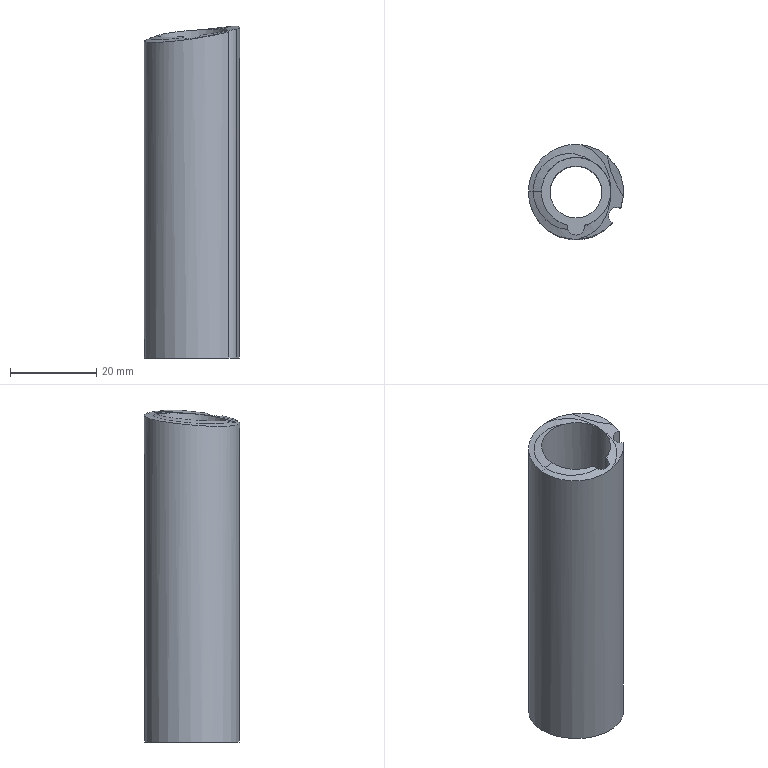Part | NX | features solid 2 | 1 solid | 14 faces | box 22 x 22.002 x 76.818 mm | volume 17878 mm3 | spline 6 | cylinder 6 | plane 2 | commonest cylinder face diameters 4 x2 12 x1 16 x1 22 x1 1640 x1
STEP:
#1=CARTESIAN_POINT('',(686.573,-10.452,-5.322));
#2=VERTEX_POINT('',#1);
#3=CARTESIAN_POINT('',(686.588,-10.686,-5.382));
#4=VERTEX_POINT('',#3);
#5=CARTESIAN_POINT('',(686.573,-10.452,-5.322));
#6=CARTESIAN_POINT('',(686.583,-10.531,-5.341));
#7=CARTESIAN_POINT('',(686.588,-10.609,-5.361));
#8=CARTESIAN_POINT('',(686.588,-10.686,-5.382));
#9=B_SPLINE_CURVE_WITH_KNOTS('',3,(#5,#6,#7,#8),.UNSPECIFIED.,.F.,.F.,(4,4),(0.00002099,0.0002621),.UNSPECIFIED.);
#10=EDGE_CURVE('',#2,#4,#9,.T.);
#11=ORIENTED_EDGE('',*,*,#10,.T.);
#12=CARTESIAN_POINT('',(686.588,-10.7,-5.386));
#13=VERTEX_POINT('',#12);
#14=CARTESIAN_POINT('',(686.588,-10.686,-5.382));
#15=CARTESIAN_POINT('',(686.588,-10.691,-5.383));
#16=CARTESIAN_POINT('',(686.588,-10.695,-5.385));
#17=CARTESIAN_POINT('',(686.588,-10.7,-5.386));
#18=B_SPLINE_CURVE_WITH_KNOTS('',3,(#14,#15,#16,#17),.UNSPECIFIED.,.F.,.F.,(4,4),(0.005452,0.005466),.UNSPECIFIED.);
#19=EDGE_CURVE('',#4,#13,#18,.T.);
#20=ORIENTED_EDGE('',*,*,#19,.T.);
#21=CARTESIAN_POINT('',(687.707,-10.069,-5.195));
#22=VERTEX_POINT('',#21);
#23=CARTESIAN_POINT('',(687.707,-10.069,-5.195));
#24=CARTESIAN_POINT('',(687.355,-10.307,-5.258));
#25=CARTESIAN_POINT('',(686.981,-10.519,-5.322));
#26=CARTESIAN_POINT('',(686.588,-10.7,-5.386));
#27=B_SPLINE_CURVE_WITH_KNOTS('',3,(#23,#24,#25,#26),.UNSPECIFIED.,.F.,.F.,(4,4),(0.3466,0.3956),.UNSPECIFIED.);
#28=EDGE_CURVE('',#22,#13,#27,.T.);
#29=ORIENTED_EDGE('',*,*,#28,.F.);
#30=CARTESIAN_POINT('',(687.707,-10.069,-5.195));
#31=CARTESIAN_POINT('',(687.34,-10.225,-5.239));
#32=CARTESIAN_POINT('',(686.962,-10.353,-5.281));
#33=CARTESIAN_POINT('',(686.573,-10.452,-5.322));
#34=B_SPLINE_CURVE_WITH_KNOTS('',3,(#30,#31,#32,#33),.UNSPECIFIED.,.F.,.F.,(4,4),(0.009294,0.0105),.UNSPECIFIED.);
#35=EDGE_CURVE('',#22,#2,#34,.T.);
#36=ORIENTED_EDGE('',*,*,#35,.T.);
#37=EDGE_LOOP('',(#11,#20,#29,#36));
#38=FACE_BOUND('',#37,.T.);
#39=CARTESIAN_POINT('',(686.515,-10.456,-5.325));
#40=CARTESIAN_POINT('',(686.529,-10.505,-5.337));
#41=CARTESIAN_POINT('',(686.542,-10.555,-5.349));
#42=CARTESIAN_POINT('',(686.555,-10.604,-5.361));
#43=CARTESIAN_POINT('',(686.568,-10.654,-5.374));
#44=CARTESIAN_POINT('',(686.581,-10.703,-5.387));
#45=CARTESIAN_POINT('',(686.761,-10.397,-5.3));
#46=CARTESIAN_POINT('',(686.775,-10.446,-5.311));
#47=CARTESIAN_POINT('',(686.79,-10.495,-5.323));
#48=CARTESIAN_POINT('',(686.805,-10.544,-5.336));
#49=CARTESIAN_POINT('',(686.82,-10.593,-5.348));
#50=CARTESIAN_POINT('',(686.834,-10.642,-5.361));
#51=CARTESIAN_POINT('',(687.004,-10.328,-5.274));
#52=CARTESIAN_POINT('',(687.02,-10.377,-5.286));
#53=CARTESIAN_POINT('',(687.036,-10.426,-5.297));
#54=CARTESIAN_POINT('',(687.053,-10.474,-5.309));
#55=CARTESIAN_POINT('',(687.069,-10.523,-5.322));
#56=CARTESIAN_POINT('',(687.085,-10.571,-5.335));
#57=CARTESIAN_POINT('',(687.244,-10.25,-5.248));
#58=CARTESIAN_POINT('',(687.261,-10.298,-5.259));
#59=CARTESIAN_POINT('',(687.279,-10.346,-5.271));
#60=CARTESIAN_POINT('',(687.297,-10.394,-5.283));
#61=CARTESIAN_POINT('',(687.315,-10.443,-5.295));
#62=CARTESIAN_POINT('',(687.333,-10.49,-5.307));
#63=CARTESIAN_POINT('',(687.48,-10.162,-5.221));
#64=CARTESIAN_POINT('',(687.5,-10.21,-5.232));
#65=CARTESIAN_POINT('',(687.519,-10.257,-5.244));
#66=CARTESIAN_POINT('',(687.538,-10.305,-5.255));
#67=CARTESIAN_POINT('',(687.558,-10.352,-5.267));
#68=CARTESIAN_POINT('',(687.577,-10.4,-5.28));
#69=CARTESIAN_POINT('',(687.713,-10.065,-5.194));
#70=CARTESIAN_POINT('',(687.734,-10.112,-5.205));
#71=CARTESIAN_POINT('',(687.755,-10.159,-5.216));
#72=CARTESIAN_POINT('',(687.776,-10.206,-5.228));
#73=CARTESIAN_POINT('',(687.797,-10.253,-5.24));
#74=CARTESIAN_POINT('',(687.818,-10.3,-5.252));
#75=B_SPLINE_SURFACE_WITH_KNOTS('',5,5,((#39,#40,#41,#42,#43,#44),(#45,#46,#47,#48,#49,#50),(#51,#52,#53,#54,#55,#56),(#57,#58,#59,#60,#61,#62),(#63,#64,#65,#66,#67,#68),(#69,#70,#71,#72,#73,#74)),.UNSPECIFIED.,.F.,.F.,.F.,(6,6),(6,6),(0.5791,0.6294),(0.4469,0.5178),.PIECEWISE_BEZIER_KNOTS.);
#76=ADVANCED_FACE('',(#38),#75,.F.);
#77=CARTESIAN_POINT('',(692.961,-9.836,-4.56));
#78=VERTEX_POINT('',#77);
#79=CARTESIAN_POINT('',(692.961,-9.836,-80.));
#80=VERTEX_POINT('',#79);
#81=CARTESIAN_POINT('',(692.961,-9.836,170.));
#82=DIRECTION('',(0.,0.,-1.));
#83=VECTOR('',#82,1000.);
#84=LINE('',#81,#83);
#85=EDGE_CURVE('',#78,#80,#84,.T.);
#86=ORIENTED_EDGE('',*,*,#85,.F.);
#87=CARTESIAN_POINT('',(684.901,-13.701,-6.131));
#88=VERTEX_POINT('',#87);
#89=CARTESIAN_POINT('',(684.948,-13.696,-6.124));
#90=CARTESIAN_POINT('',(688.008,-13.596,-5.653));
#91=CARTESIAN_POINT('',(690.985,-12.155,-5.066));
#92=CARTESIAN_POINT('',(692.961,-9.836,-4.56));
#93=B_SPLINE_CURVE_WITH_KNOTS('',3,(#89,#90,#91,#92),.UNSPECIFIED.,.F.,.F.,(4,4),(0.01762,0.02686),.UNSPECIFIED.);
#94=EDGE_CURVE('',#88,#78,#93,.T.);
#95=ORIENTED_EDGE('',*,*,#94,.F.);
#96=CARTESIAN_POINT('',(673.59,-2.498,-6.658));
#97=VERTEX_POINT('',#96);
#98=CARTESIAN_POINT('',(673.59,-2.498,-6.658));
#99=CARTESIAN_POINT('',(673.535,-5.487,-6.917));
#100=CARTESIAN_POINT('',(675.984,-11.422,-7.155));
#101=CARTESIAN_POINT('',(681.928,-13.779,-6.586));
#102=CARTESIAN_POINT('',(684.89,-13.698,-6.132));
#103=B_SPLINE_CURVE_WITH_KNOTS('',3,(#98,#99,#100,#101,#102),.UNSPECIFIED.,.F.,.F.,(4,1,4),(0.,0.008898,0.0178),.UNSPECIFIED.);
#104=EDGE_CURVE('',#97,#88,#103,.T.);
#105=ORIENTED_EDGE('',*,*,#104,.F.);
#106=CARTESIAN_POINT('',(685.747,8.237,-4.236));
#107=VERTEX_POINT('',#106);
#108=CARTESIAN_POINT('',(673.59,-2.498,-6.658));
#109=CARTESIAN_POINT('',(673.647,0.5842,-6.392));
#110=CARTESIAN_POINT('',(676.467,6.538,-5.598));
#111=CARTESIAN_POINT('',(682.699,8.559,-4.676));
#112=CARTESIAN_POINT('',(685.745,8.237,-4.237));
#113=B_SPLINE_CURVE_WITH_KNOTS('',3,(#108,#109,#110,#111,#112),.UNSPECIFIED.,.F.,.F.,(4,1,4),(0.,0.009181,0.01836),.UNSPECIFIED.);
#114=EDGE_CURVE('',#97,#107,#113,.T.);
#115=ORIENTED_EDGE('',*,*,#114,.T.);
#116=CARTESIAN_POINT('',(691.785,5.616,-3.502));
#117=VERTEX_POINT('',#116);
#118=CARTESIAN_POINT('',(691.783,5.619,-3.503));
#119=CARTESIAN_POINT('',(690.087,7.085,-3.656));
#120=CARTESIAN_POINT('',(687.953,8.002,-3.918));
#121=CARTESIAN_POINT('',(685.754,8.236,-4.235));
#122=B_SPLINE_CURVE_WITH_KNOTS('',3,(#118,#119,#120,#121),.UNSPECIFIED.,.F.,.F.,(4,4),(0.04406,0.05075),.UNSPECIFIED.);
#123=EDGE_CURVE('',#117,#107,#122,.T.);
#124=ORIENTED_EDGE('',*,*,#123,.F.);
#125=CARTESIAN_POINT('',(695.532,-3.818,-3.655));
#126=VERTEX_POINT('',#125);
#127=CARTESIAN_POINT('',(691.788,5.614,-3.502));
#128=CARTESIAN_POINT('',(693.13,4.452,-3.381));
#129=CARTESIAN_POINT('',(695.206,1.508,-2.937));
#130=CARTESIAN_POINT('',(695.711,-2.052,-3.483));
#131=CARTESIAN_POINT('',(695.532,-3.814,-3.655));
#132=B_SPLINE_CURVE_WITH_KNOTS('',3,(#127,#128,#129,#130,#131),.UNSPECIFIED.,.F.,.F.,(4,1,4),(0.,0.005263,0.01053),.UNSPECIFIED.);
#133=EDGE_CURVE('',#117,#126,#132,.T.);
#134=ORIENTED_EDGE('',*,*,#133,.T.);
#135=CARTESIAN_POINT('',(694.953,-6.386,-3.958));
#136=VERTEX_POINT('',#135);
#137=CARTESIAN_POINT('',(694.953,-6.386,-3.958));
#138=CARTESIAN_POINT('',(695.246,-5.562,-3.843));
#139=CARTESIAN_POINT('',(695.441,-4.706,-3.742));
#140=CARTESIAN_POINT('',(695.531,-3.822,-3.655));
#141=B_SPLINE_CURVE_WITH_KNOTS('',3,(#137,#138,#139,#140),.UNSPECIFIED.,.F.,.F.,(4,4),(0.03089,0.03354),.UNSPECIFIED.);
#142=EDGE_CURVE('',#136,#126,#141,.T.);
#143=ORIENTED_EDGE('',*,*,#142,.F.);
#144=CARTESIAN_POINT('',(694.953,-6.386,-80.));
#145=VERTEX_POINT('',#144);
#146=CARTESIAN_POINT('',(694.953,-6.386,170.));
#147=DIRECTION('',(0.,0.,-1.));
#148=VECTOR('',#147,1000.);
#149=LINE('',#146,#148);
#150=EDGE_CURVE('',#145,#136,#149,.F.);
#151=ORIENTED_EDGE('',*,*,#150,.F.);
#152=CARTESIAN_POINT('',(684.588,-2.702,-80.));
#153=DIRECTION('',(0.,0.,1.));
#154=DIRECTION('',(1.,0.,0.));
#155=AXIS2_PLACEMENT_3D('',#152,#153,#154);
#156=CIRCLE('',#155,11.);
#157=EDGE_CURVE('',#145,#80,#156,.T.);
#158=ORIENTED_EDGE('',*,*,#157,.T.);
#159=EDGE_LOOP('',(#86,#95,#105,#115,#124,#134,#143,#151,#158));
#160=FACE_BOUND('',#159,.T.);
#161=CARTESIAN_POINT('',(684.588,-2.702,27.));
#162=DIRECTION('',(0.,0.,-1.));
#163=DIRECTION('',(-1.,0.,0.));
#164=AXIS2_PLACEMENT_3D('',#161,#162,#163);
#165=CYLINDRICAL_SURFACE('',#164,11.);
#166=ADVANCED_FACE('',(#160),#165,.T.);
#167=CARTESIAN_POINT('',(690.588,-2.702,-80.));
#168=VERTEX_POINT('',#167);
#169=CARTESIAN_POINT('',(684.588,-2.702,-80.));
#170=DIRECTION('',(0.,0.,1.));
#171=DIRECTION('',(1.,0.,0.));
#172=AXIS2_PLACEMENT_3D('',#169,#170,#171);
#173=CIRCLE('',#172,6.);
#174=EDGE_CURVE('',#168,#168,#173,.T.);
#175=ORIENTED_EDGE('',*,*,#174,.T.);
#176=EDGE_LOOP('',(#175));
#177=FACE_BOUND('',#176,.T.);
#178=CARTESIAN_POINT('',(694.115,-8.202,-80.));
#179=DIRECTION('',(0.,0.,1.));
#180=DIRECTION('',(0.866,-0.5,0.));
#181=AXIS2_PLACEMENT_3D('',#178,#179,#180);
#182=CIRCLE('',#181,2.);
#183=EDGE_CURVE('',#145,#80,#182,.T.);
#184=ORIENTED_EDGE('',*,*,#183,.T.);
#185=ORIENTED_EDGE('',*,*,#157,.F.);
#186=EDGE_LOOP('',(#184,#185));
#187=FACE_BOUND('',#186,.T.);
#188=CARTESIAN_POINT('',(-628.999,-86.749,-80.));
#189=DIRECTION('',(0.,0.,1.));
#190=DIRECTION('',(1.,0.,0.));
#191=AXIS2_PLACEMENT_3D('',#188,#189,#190);
#192=PLANE('',#191);
#193=ADVANCED_FACE('',(#177,#187),#192,.F.);
#194=ORIENTED_EDGE('',*,*,#94,.T.);
#195=CARTESIAN_POINT('',(692.961,-9.836,-4.56));
#196=CARTESIAN_POINT('',(692.558,-9.552,-4.602));
#197=CARTESIAN_POINT('',(691.968,-8.66,-4.625));
#198=CARTESIAN_POINT('',(692.228,-7.09,-4.457));
#199=CARTESIAN_POINT('',(693.458,-6.116,-4.18));
#200=CARTESIAN_POINT('',(694.506,-6.18,-4.014));
#201=CARTESIAN_POINT('',(694.953,-6.386,-3.958));
#202=B_SPLINE_CURVE_WITH_KNOTS('',3,(#195,#196,#197,#198,#199,#200,#201),.UNSPECIFIED.,.F.,.F.,(4,1,1,1,4),(0.003125,0.00461,0.006094,0.007579,0.009063),.UNSPECIFIED.);
#203=EDGE_CURVE('',#78,#136,#202,.T.);
#204=ORIENTED_EDGE('',*,*,#203,.T.);
#205=ORIENTED_EDGE('',*,*,#142,.T.);
#206=CARTESIAN_POINT('',(691.783,5.616,-3.503));
#207=CARTESIAN_POINT('',(692.343,2.264,-3.684));
#208=CARTESIAN_POINT('',(693.654,-1.017,-3.738));
#209=CARTESIAN_POINT('',(695.53,-3.82,-3.656));
#210=B_SPLINE_CURVE_WITH_KNOTS('',3,(#206,#207,#208,#209),.UNSPECIFIED.,.F.,.F.,(4,4),(0.1057,0.3726),.UNSPECIFIED.);
#211=EDGE_CURVE('',#126,#117,#210,.F.);
#212=ORIENTED_EDGE('',*,*,#211,.T.);
#213=ORIENTED_EDGE('',*,*,#123,.T.);
#214=CARTESIAN_POINT('',(692.623,-2.801,-4.047));
#215=VERTEX_POINT('',#214);
#216=CARTESIAN_POINT('',(685.75,8.237,-4.236));
#217=CARTESIAN_POINT('',(686.39,8.019,-4.156));
#218=CARTESIAN_POINT('',(687.294,7.605,-4.05));
#219=CARTESIAN_POINT('',(688.457,6.826,-3.932));
#220=CARTESIAN_POINT('',(689.404,6.048,-3.846));
#221=CARTESIAN_POINT('',(690.246,5.136,-3.787));
#222=CARTESIAN_POINT('',(690.868,4.228,-3.761));
#223=CARTESIAN_POINT('',(691.181,3.695,-3.754));
#224=CARTESIAN_POINT('',(691.498,3.099,-3.751));
#225=CARTESIAN_POINT('',(691.949,2.052,-3.764));
#226=CARTESIAN_POINT('',(692.483,0.08758,-3.836));
#227=CARTESIAN_POINT('',(692.637,-1.596,-3.948));
#228=CARTESIAN_POINT('',(692.623,-2.801,-4.047));
#229=B_SPLINE_CURVE_WITH_KNOTS('',3,(#216,#217,#218,#219,#220,#221,#222,#223,#224,#225,#226,#227,#228),.UNSPECIFIED.,.F.,.F.,(4,1,1,1,1,1,1,1,1,1,4),(0.5367,0.5946,0.6236,0.6525,0.7104,0.7394,0.7539,0.7683,0.8263,0.8842,1.),.UNSPECIFIED.);
#230=EDGE_CURVE('',#107,#215,#229,.T.);
#231=ORIENTED_EDGE('',*,*,#230,.T.);
#232=CARTESIAN_POINT('',(684.912,-13.704,-6.13));
#233=CARTESIAN_POINT('',(685.602,-13.549,-6.013));
#234=CARTESIAN_POINT('',(686.915,-13.103,-5.777));
#235=CARTESIAN_POINT('',(688.718,-11.987,-5.408));
#236=CARTESIAN_POINT('',(689.847,-10.911,-5.144));
#237=CARTESIAN_POINT('',(690.532,-10.04,-4.965));
#238=CARTESIAN_POINT('',(690.902,-9.484,-4.862));
#239=CARTESIAN_POINT('',(691.19,-9.002,-4.777));
#240=CARTESIAN_POINT('',(691.46,-8.481,-4.692));
#241=CARTESIAN_POINT('',(691.867,-7.54,-4.551));
#242=CARTESIAN_POINT('',(692.408,-5.789,-4.323));
#243=CARTESIAN_POINT('',(692.609,-4.055,-4.15));
#244=CARTESIAN_POINT('',(692.623,-2.801,-4.047));
#245=B_SPLINE_CURVE_WITH_KNOTS('',3,(#232,#233,#234,#235,#236,#237,#238,#239,#240,#241,#242,#243,#244),.UNSPECIFIED.,.F.,.F.,(4,1,1,1,1,1,1,1,1,1,4),(0.5156,0.5762,0.6367,0.6973,0.7275,0.7427,0.7578,0.7881,0.8184,0.8789,1.),.UNSPECIFIED.);
#246=EDGE_CURVE('',#88,#215,#245,.T.);
#247=ORIENTED_EDGE('',*,*,#246,.F.);
#248=EDGE_LOOP('',(#194,#204,#205,#212,#213,#231,#247));
#249=FACE_BOUND('',#248,.T.);
#250=CARTESIAN_POINT('',(561.704,-30.67,805.818));
#251=DIRECTION('',(0.02304,-0.9968,-0.07674));
#252=DIRECTION('',(0.9976,0.02799,-0.06404));
#253=AXIS2_PLACEMENT_3D('',#250,#251,#252);
#254=CYLINDRICAL_SURFACE('',#253,820.);
#255=ADVANCED_FACE('',(#249),#254,.F.);
#256=ORIENTED_EDGE('',*,*,#211,.F.);
#257=ORIENTED_EDGE('',*,*,#133,.F.);
#258=EDGE_LOOP('',(#256,#257));
#259=FACE_BOUND('',#258,.T.);
#260=CARTESIAN_POINT('',(695.568,-3.868,-3.653));
#261=CARTESIAN_POINT('',(695.914,-3.635,-3.577));
#262=CARTESIAN_POINT('',(696.256,-3.405,-3.479));
#263=CARTESIAN_POINT('',(696.594,-3.177,-3.36));
#264=CARTESIAN_POINT('',(696.925,-2.952,-3.219));
#265=CARTESIAN_POINT('',(697.249,-2.732,-3.057));
#266=CARTESIAN_POINT('',(694.938,-2.931,-3.681));
#267=CARTESIAN_POINT('',(695.294,-2.716,-3.606));
#268=CARTESIAN_POINT('',(695.647,-2.503,-3.508));
#269=CARTESIAN_POINT('',(695.995,-2.292,-3.388));
#270=CARTESIAN_POINT('',(696.336,-2.085,-3.248));
#271=CARTESIAN_POINT('',(696.67,-1.882,-3.086));
#272=CARTESIAN_POINT('',(694.361,-1.956,-3.697));
#273=CARTESIAN_POINT('',(694.727,-1.759,-3.621));
#274=CARTESIAN_POINT('',(695.089,-1.564,-3.524));
#275=CARTESIAN_POINT('',(695.446,-1.371,-3.405));
#276=CARTESIAN_POINT('',(695.797,-1.181,-3.265));
#277=CARTESIAN_POINT('',(696.14,-0.9951,-3.104));
#278=CARTESIAN_POINT('',(693.842,-0.9469,-3.7));
#279=CARTESIAN_POINT('',(694.215,-0.7679,-3.625));
#280=CARTESIAN_POINT('',(694.586,-0.5907,-3.528));
#281=CARTESIAN_POINT('',(694.951,-0.4159,-3.409));
#282=CARTESIAN_POINT('',(695.31,-0.2441,-3.27));
#283=CARTESIAN_POINT('',(695.662,-0.07604,-3.11));
#284=CARTESIAN_POINT('',(693.03,0.8862,-3.684));
#285=CARTESIAN_POINT('',(693.417,1.032,-3.609));
#286=CARTESIAN_POINT('',(693.8,1.177,-3.513));
#287=CARTESIAN_POINT('',(694.179,1.319,-3.396));
#288=CARTESIAN_POINT('',(694.55,1.459,-3.258));
#289=CARTESIAN_POINT('',(694.915,1.595,-3.099));
#290=CARTESIAN_POINT('',(692.413,2.795,-3.629));
#291=CARTESIAN_POINT('',(692.809,2.908,-3.556));
#292=CARTESIAN_POINT('',(693.202,3.019,-3.462));
#293=CARTESIAN_POINT('',(693.59,3.128,-3.346));
#294=CARTESIAN_POINT('',(693.971,3.234,-3.21));
#295=CARTESIAN_POINT('',(694.345,3.337,-3.053));
#296=CARTESIAN_POINT('',(692.182,3.634,-3.599));
#297=CARTESIAN_POINT('',(692.582,3.732,-3.526));
#298=CARTESIAN_POINT('',(692.979,3.829,-3.433));
#299=CARTESIAN_POINT('',(693.37,3.923,-3.318));
#300=CARTESIAN_POINT('',(693.755,4.015,-3.182));
#301=CARTESIAN_POINT('',(694.133,4.104,-3.026));
#302=CARTESIAN_POINT('',(691.975,4.55,-3.558));
#303=CARTESIAN_POINT('',(692.378,4.632,-3.487));
#304=CARTESIAN_POINT('',(692.778,4.712,-3.394));
#305=CARTESIAN_POINT('',(693.172,4.791,-3.28));
#306=CARTESIAN_POINT('',(693.561,4.867,-3.145));
#307=CARTESIAN_POINT('',(693.942,4.94,-2.99));
#308=CARTESIAN_POINT('',(691.812,5.474,-3.51));
#309=CARTESIAN_POINT('',(692.218,5.54,-3.439));
#310=CARTESIAN_POINT('',(692.62,5.604,-3.347));
#311=CARTESIAN_POINT('',(693.017,5.667,-3.235));
#312=CARTESIAN_POINT('',(693.408,5.727,-3.101));
#313=CARTESIAN_POINT('',(693.791,5.785,-2.947));
#314=CARTESIAN_POINT('',(691.8,5.542,-3.506));
#315=CARTESIAN_POINT('',(692.206,5.607,-3.436));
#316=CARTESIAN_POINT('',(692.609,5.67,-3.344));
#317=CARTESIAN_POINT('',(693.006,5.731,-3.231));
#318=CARTESIAN_POINT('',(693.397,5.79,-3.098));
#319=CARTESIAN_POINT('',(693.781,5.847,-2.944));
#320=CARTESIAN_POINT('',(691.789,5.61,-3.502));
#321=CARTESIAN_POINT('',(692.195,5.673,-3.432));
#322=CARTESIAN_POINT('',(692.597,5.735,-3.34));
#323=CARTESIAN_POINT('',(692.995,5.795,-3.228));
#324=CARTESIAN_POINT('',(693.386,5.853,-3.094));
#325=CARTESIAN_POINT('',(693.77,5.909,-2.941));
#326=CARTESIAN_POINT('',(691.778,5.678,-3.499));
#327=CARTESIAN_POINT('',(692.184,5.74,-3.429));
#328=CARTESIAN_POINT('',(692.587,5.801,-3.337));
#329=CARTESIAN_POINT('',(692.984,5.86,-3.224));
#330=CARTESIAN_POINT('',(693.376,5.916,-3.091));
#331=CARTESIAN_POINT('',(693.76,5.971,-2.937));
#332=B_SPLINE_SURFACE_WITH_KNOTS('',5,5,((#260,#261,#262,#263,#264,#265),(#266,#267,#268,#269,#270,#271),(#272,#273,#274,#275,#276,#277),(#278,#279,#280,#281,#282,#283),(#284,#285,#286,#287,#288,#289),(#290,#291,#292,#293,#294,#295),(#296,#297,#298,#299,#300,#301),(#302,#303,#304,#305,#306,#307),(#308,#309,#310,#311,#312,#313),(#314,#315,#316,#317,#318,#319),(#320,#321,#322,#323,#324,#325),(#326,#327,#328,#329,#330,#331)),.UNSPECIFIED.,.F.,.F.,.F.,(6,3,3,6),(6,6),(0.6261,0.7739,0.887,0.8959),(0.,0.4938),.UNSPECIFIED.);
#333=ADVANCED_FACE('',(#259),#332,.F.);
#334=CARTESIAN_POINT('',(674.688,-2.535,-6.203));
#335=VERTEX_POINT('',#334);
#336=CARTESIAN_POINT('',(674.688,-2.535,-6.203));
#337=CARTESIAN_POINT('',(674.331,-2.521,-6.376));
#338=CARTESIAN_POINT('',(673.965,-2.509,-6.528));
#339=CARTESIAN_POINT('',(673.59,-2.498,-6.658));
#340=B_SPLINE_CURVE_WITH_KNOTS('',3,(#336,#337,#338,#339),.UNSPECIFIED.,.F.,.F.,(4,4),(0.,0.3711),.UNSPECIFIED.);
#341=EDGE_CURVE('',#335,#97,#340,.T.);
#342=ORIENTED_EDGE('',*,*,#341,.F.);
#343=CARTESIAN_POINT('',(687.878,4.59,-3.984));
#344=VERTEX_POINT('',#343);
#345=CARTESIAN_POINT('',(687.878,4.59,-3.984));
#346=CARTESIAN_POINT('',(686.719,5.44,-4.06));
#347=CARTESIAN_POINT('',(683.861,6.559,-4.333));
#348=CARTESIAN_POINT('',(679.15,5.648,-5.001));
#349=CARTESIAN_POINT('',(675.576,2.281,-5.709));
#350=CARTESIAN_POINT('',(674.69,-0.9257,-6.073));
#351=CARTESIAN_POINT('',(674.688,-2.535,-6.203));
#352=B_SPLINE_CURVE_WITH_KNOTS('',3,(#345,#346,#347,#348,#349,#350,#351),.UNSPECIFIED.,.F.,.F.,(4,1,1,1,4),(0.3426,0.5069,0.6713,0.8356,1.),.UNSPECIFIED.);
#353=EDGE_CURVE('',#344,#335,#352,.T.);
#354=ORIENTED_EDGE('',*,*,#353,.F.);
#355=CARTESIAN_POINT('',(692.588,-2.8,-4.053));
#356=VERTEX_POINT('',#355);
#357=CARTESIAN_POINT('',(687.878,4.59,-3.984));
#358=CARTESIAN_POINT('',(689.299,3.949,-3.92));
#359=CARTESIAN_POINT('',(691.711,1.852,-3.826));
#360=CARTESIAN_POINT('',(692.607,-1.245,-3.924));
#361=CARTESIAN_POINT('',(692.588,-2.8,-4.053));
#362=B_SPLINE_CURVE_WITH_KNOTS('',3,(#357,#358,#359,#360,#361),.UNSPECIFIED.,.F.,.F.,(4,1,4),(0.,0.004613,0.009227),.UNSPECIFIED.);
#363=EDGE_CURVE('',#344,#356,#362,.T.);
#364=ORIENTED_EDGE('',*,*,#363,.T.);
#365=CARTESIAN_POINT('',(692.623,-2.801,-4.047));
#366=CARTESIAN_POINT('',(692.611,-2.8,-4.049));
#367=CARTESIAN_POINT('',(692.6,-2.8,-4.051));
#368=CARTESIAN_POINT('',(692.588,-2.8,-4.053));
#369=B_SPLINE_CURVE_WITH_KNOTS('',3,(#365,#366,#367,#368),.UNSPECIFIED.,.F.,.F.,(4,4),(0.,0.02906),.UNSPECIFIED.);
#370=EDGE_CURVE('',#215,#356,#369,.T.);
#371=ORIENTED_EDGE('',*,*,#370,.F.);
#372=ORIENTED_EDGE('',*,*,#230,.F.);
#373=ORIENTED_EDGE('',*,*,#114,.F.);
#374=EDGE_LOOP('',(#342,#354,#364,#371,#372,#373));
#375=FACE_BOUND('',#374,.T.);
#376=CARTESIAN_POINT('',(671.633,-2.461,-7.124));
#377=CARTESIAN_POINT('',(672.268,-2.468,-7.039));
#378=CARTESIAN_POINT('',(672.897,-2.479,-6.903));
#379=CARTESIAN_POINT('',(673.513,-2.494,-6.717));
#380=CARTESIAN_POINT('',(674.112,-2.513,-6.483));
#381=CARTESIAN_POINT('',(674.688,-2.535,-6.203));
#382=CARTESIAN_POINT('',(671.634,-1.201,-7.023));
#383=CARTESIAN_POINT('',(672.269,-1.276,-6.943));
#384=CARTESIAN_POINT('',(672.898,-1.356,-6.813));
#385=CARTESIAN_POINT('',(673.514,-1.439,-6.632));
#386=CARTESIAN_POINT('',(674.113,-1.524,-6.403));
#387=CARTESIAN_POINT('',(674.689,-1.612,-6.128));
#388=CARTESIAN_POINT('',(671.804,0.0567,-6.899));
#389=CARTESIAN_POINT('',(672.429,-0.08687,-6.826));
#390=CARTESIAN_POINT('',(673.047,-0.2345,-6.703));
#391=CARTESIAN_POINT('',(673.653,-0.3849,-6.529));
#392=CARTESIAN_POINT('',(674.242,-0.5369,-6.308));
#393=CARTESIAN_POINT('',(674.808,-0.6891,-6.04));
#394=CARTESIAN_POINT('',(672.143,1.281,-6.755));
#395=CARTESIAN_POINT('',(672.747,1.071,-6.69));
#396=CARTESIAN_POINT('',(673.344,0.8575,-6.575));
#397=CARTESIAN_POINT('',(673.93,0.6416,-6.41));
#398=CARTESIAN_POINT('',(674.498,0.4254,-6.198));
#399=CARTESIAN_POINT('',(675.045,0.2106,-5.939));
#400=CARTESIAN_POINT('',(673.582,4.609,-6.294));
#401=CARTESIAN_POINT('',(674.097,4.223,-6.254));
#402=CARTESIAN_POINT('',(674.605,3.833,-6.166));
#403=CARTESIAN_POINT('',(675.102,3.442,-6.03));
#404=CARTESIAN_POINT('',(675.585,3.054,-5.847));
#405=CARTESIAN_POINT('',(676.049,2.671,-5.62));
#406=CARTESIAN_POINT('',(676.202,7.164,-5.726));
#407=CARTESIAN_POINT('',(676.558,6.655,-5.717));
#408=CARTESIAN_POINT('',(676.907,6.141,-5.663));
#409=CARTESIAN_POINT('',(677.247,5.629,-5.565));
#410=CARTESIAN_POINT('',(677.576,5.12,-5.422));
#411=CARTESIAN_POINT('',(677.891,4.619,-5.238));
#412=CARTESIAN_POINT('',(678.304,8.32,-5.337));
#413=CARTESIAN_POINT('',(678.534,7.765,-5.348));
#414=CARTESIAN_POINT('',(678.758,7.206,-5.317));
#415=CARTESIAN_POINT('',(678.974,6.649,-5.245));
#416=CARTESIAN_POINT('',(679.182,6.095,-5.132));
#417=CARTESIAN_POINT('',(679.379,5.55,-4.979));
#418=CARTESIAN_POINT('',(682.432,9.268,-4.659));
#419=CARTESIAN_POINT('',(682.43,8.708,-4.704));
#420=CARTESIAN_POINT('',(682.423,8.145,-4.713));
#421=CARTESIAN_POINT('',(682.411,7.582,-4.687));
#422=CARTESIAN_POINT('',(682.394,7.023,-4.625));
#423=CARTESIAN_POINT('',(682.372,6.471,-4.529));
#424=CARTESIAN_POINT('',(686.302,8.282,-4.151));
#425=CARTESIAN_POINT('',(686.119,7.828,-4.215));
#426=CARTESIAN_POINT('',(685.932,7.372,-4.251));
#427=CARTESIAN_POINT('',(685.742,6.916,-4.258));
#428=CARTESIAN_POINT('',(685.549,6.461,-4.237));
#429=CARTESIAN_POINT('',(685.354,6.011,-4.187));
#430=CARTESIAN_POINT('',(687.873,7.465,-3.973));
#431=CARTESIAN_POINT('',(687.628,7.078,-4.042));
#432=CARTESIAN_POINT('',(687.379,6.689,-4.086));
#433=CARTESIAN_POINT('',(687.127,6.299,-4.105));
#434=CARTESIAN_POINT('',(686.873,5.911,-4.098));
#435=CARTESIAN_POINT('',(686.619,5.525,-4.065));
#436=CARTESIAN_POINT('',(689.86,5.811,-3.794));
#437=CARTESIAN_POINT('',(689.558,5.537,-3.864));
#438=CARTESIAN_POINT('',(689.253,5.26,-3.913));
#439=CARTESIAN_POINT('',(688.946,4.983,-3.943));
#440=CARTESIAN_POINT('',(688.638,4.706,-3.951));
#441=CARTESIAN_POINT('',(688.33,4.43,-3.939));
#442=CARTESIAN_POINT('',(691.158,3.833,-3.747));
#443=CARTESIAN_POINT('',(690.849,3.66,-3.81));
#444=CARTESIAN_POINT('',(690.538,3.485,-3.858));
#445=CARTESIAN_POINT('',(690.225,3.31,-3.889));
#446=CARTESIAN_POINT('',(689.911,3.134,-3.905));
#447=CARTESIAN_POINT('',(689.597,2.958,-3.905));
#448=CARTESIAN_POINT('',(691.529,3.112,-3.746));
#449=CARTESIAN_POINT('',(691.223,2.972,-3.806));
#450=CARTESIAN_POINT('',(690.915,2.83,-3.852));
#451=CARTESIAN_POINT('',(690.605,2.688,-3.884));
#452=CARTESIAN_POINT('',(690.295,2.545,-3.901));
#453=CARTESIAN_POINT('',(689.984,2.402,-3.904));
#454=CARTESIAN_POINT('',(691.981,1.987,-3.764));
#455=CARTESIAN_POINT('',(691.685,1.891,-3.819));
#456=CARTESIAN_POINT('',(691.388,1.794,-3.862));
#457=CARTESIAN_POINT('',(691.089,1.697,-3.893));
#458=CARTESIAN_POINT('',(690.79,1.599,-3.912));
#459=CARTESIAN_POINT('',(690.491,1.5,-3.918));
#460=CARTESIAN_POINT('',(692.269,0.873,-3.808));
#461=CARTESIAN_POINT('',(691.989,0.8111,-3.858));
#462=CARTESIAN_POINT('',(691.707,0.7484,-3.897));
#463=CARTESIAN_POINT('',(691.424,0.6849,-3.926));
#464=CARTESIAN_POINT('',(691.14,0.6208,-3.945));
#465=CARTESIAN_POINT('',(690.856,0.5562,-3.953));
#466=CARTESIAN_POINT('',(692.353,0.4798,-3.826));
#467=CARTESIAN_POINT('',(692.078,0.4285,-3.874));
#468=CARTESIAN_POINT('',(691.802,0.3765,-3.913));
#469=CARTESIAN_POINT('',(691.524,0.3237,-3.941));
#470=CARTESIAN_POINT('',(691.246,0.2703,-3.96));
#471=CARTESIAN_POINT('',(690.968,0.2164,-3.968));
#472=CARTESIAN_POINT('',(692.466,-0.1667,-3.86));
#473=CARTESIAN_POINT('',(692.2,-0.2025,-3.906));
#474=CARTESIAN_POINT('',(691.933,-0.2389,-3.942));
#475=CARTESIAN_POINT('',(691.664,-0.2761,-3.97));
#476=CARTESIAN_POINT('',(691.396,-0.3139,-3.988));
#477=CARTESIAN_POINT('',(691.126,-0.3523,-3.997));
#478=CARTESIAN_POINT('',(692.539,-0.8027,-3.899));
#479=CARTESIAN_POINT('',(692.281,-0.8261,-3.943));
#480=CARTESIAN_POINT('',(692.022,-0.8502,-3.978));
#481=CARTESIAN_POINT('',(691.762,-0.875,-4.004));
#482=CARTESIAN_POINT('',(691.501,-0.9004,-4.022));
#483=CARTESIAN_POINT('',(691.24,-0.9264,-4.031));
#484=CARTESIAN_POINT('',(692.563,-1.055,-3.916));
#485=CARTESIAN_POINT('',(692.308,-1.074,-3.958));
#486=CARTESIAN_POINT('',(692.051,-1.093,-3.993));
#487=CARTESIAN_POINT('',(691.794,-1.113,-4.019));
#488=CARTESIAN_POINT('',(691.536,-1.134,-4.037));
#489=CARTESIAN_POINT('',(691.278,-1.156,-4.046));
#490=CARTESIAN_POINT('',(692.591,-1.43,-3.942));
#491=CARTESIAN_POINT('',(692.34,-1.443,-3.983));
#492=CARTESIAN_POINT('',(692.087,-1.457,-4.017));
#493=CARTESIAN_POINT('',(691.834,-1.471,-4.042));
#494=CARTESIAN_POINT('',(691.579,-1.485,-4.06));
#495=CARTESIAN_POINT('',(691.325,-1.501,-4.069));
#496=CARTESIAN_POINT('',(692.609,-1.803,-3.969));
#497=CARTESIAN_POINT('',(692.36,-1.811,-4.009));
#498=CARTESIAN_POINT('',(692.11,-1.819,-4.042));
#499=CARTESIAN_POINT('',(691.86,-1.827,-4.067));
#500=CARTESIAN_POINT('',(691.609,-1.837,-4.084));
#501=CARTESIAN_POINT('',(691.357,-1.846,-4.094));
#502=CARTESIAN_POINT('',(692.614,-1.927,-3.978));
#503=CARTESIAN_POINT('',(692.366,-1.933,-4.018));
#504=CARTESIAN_POINT('',(692.117,-1.939,-4.051));
#505=CARTESIAN_POINT('',(691.867,-1.946,-4.076));
#506=CARTESIAN_POINT('',(691.617,-1.954,-4.093));
#507=CARTESIAN_POINT('',(691.366,-1.962,-4.102));
#508=CARTESIAN_POINT('',(692.62,-2.137,-3.994));
#509=CARTESIAN_POINT('',(692.373,-2.14,-4.034));
#510=CARTESIAN_POINT('',(692.126,-2.143,-4.066));
#511=CARTESIAN_POINT('',(691.877,-2.147,-4.091));
#512=CARTESIAN_POINT('',(691.628,-2.152,-4.108));
#513=CARTESIAN_POINT('',(691.378,-2.157,-4.117));
#514=CARTESIAN_POINT('',(692.623,-2.346,-4.01));
#515=CARTESIAN_POINT('',(692.378,-2.346,-4.05));
#516=CARTESIAN_POINT('',(692.131,-2.347,-4.082));
#517=CARTESIAN_POINT('',(691.883,-2.348,-4.106));
#518=CARTESIAN_POINT('',(691.635,-2.35,-4.123));
#519=CARTESIAN_POINT('',(691.386,-2.352,-4.132));
#520=CARTESIAN_POINT('',(692.624,-2.431,-4.017));
#521=CARTESIAN_POINT('',(692.379,-2.43,-4.057));
#522=CARTESIAN_POINT('',(692.132,-2.43,-4.088));
#523=CARTESIAN_POINT('',(691.885,-2.43,-4.113));
#524=CARTESIAN_POINT('',(691.637,-2.431,-4.129));
#525=CARTESIAN_POINT('',(691.389,-2.432,-4.138));
#526=CARTESIAN_POINT('',(692.625,-2.555,-4.027));
#527=CARTESIAN_POINT('',(692.38,-2.552,-4.066));
#528=CARTESIAN_POINT('',(692.134,-2.55,-4.098));
#529=CARTESIAN_POINT('',(691.887,-2.549,-4.122));
#530=CARTESIAN_POINT('',(691.639,-2.548,-4.138));
#531=CARTESIAN_POINT('',(691.391,-2.547,-4.147));
#532=CARTESIAN_POINT('',(692.624,-2.678,-4.037));
#533=CARTESIAN_POINT('',(692.38,-2.674,-4.076));
#534=CARTESIAN_POINT('',(692.134,-2.67,-4.108));
#535=CARTESIAN_POINT('',(691.887,-2.667,-4.132));
#536=CARTESIAN_POINT('',(691.639,-2.665,-4.148));
#537=CARTESIAN_POINT('',(691.392,-2.663,-4.156));
#538=CARTESIAN_POINT('',(692.624,-2.725,-4.041));
#539=CARTESIAN_POINT('',(692.379,-2.721,-4.08));
#540=CARTESIAN_POINT('',(692.133,-2.716,-4.111));
#541=CARTESIAN_POINT('',(691.887,-2.713,-4.135));
#542=CARTESIAN_POINT('',(691.639,-2.71,-4.151));
#543=CARTESIAN_POINT('',(691.392,-2.707,-4.16));
#544=CARTESIAN_POINT('',(692.624,-2.763,-4.044));
#545=CARTESIAN_POINT('',(692.379,-2.758,-4.083));
#546=CARTESIAN_POINT('',(692.133,-2.753,-4.114));
#547=CARTESIAN_POINT('',(691.887,-2.749,-4.138));
#548=CARTESIAN_POINT('',(691.639,-2.745,-4.154));
#549=CARTESIAN_POINT('',(691.392,-2.742,-4.163));
#550=CARTESIAN_POINT('',(692.623,-2.801,-4.047));
#551=CARTESIAN_POINT('',(692.379,-2.795,-4.086));
#552=CARTESIAN_POINT('',(692.133,-2.79,-4.117));
#553=CARTESIAN_POINT('',(691.886,-2.785,-4.141));
#554=CARTESIAN_POINT('',(691.639,-2.781,-4.157));
#555=CARTESIAN_POINT('',(691.391,-2.778,-4.166));
#556=B_SPLINE_SURFACE_WITH_KNOTS('',5,5,((#376,#377,#378,#379,#380,#381),(#382,#383,#384,#385,#386,#387),(#388,#389,#390,#391,#392,#393),(#394,#395,#396,#397,#398,#399),(#400,#401,#402,#403,#404,#405),(#406,#407,#408,#409,#410,#411),(#412,#413,#414,#415,#416,#417),(#418,#419,#420,#421,#422,#423),(#424,#425,#426,#427,#428,#429),(#430,#431,#432,#433,#434,#435),(#436,#437,#438,#439,#440,#441),(#442,#443,#444,#445,#446,#447),(#448,#449,#450,#451,#452,#453),(#454,#455,#456,#457,#458,#459),(#460,#461,#462,#463,#464,#465),(#466,#467,#468,#469,#470,#471),(#472,#473,#474,#475,#476,#477),(#478,#479,#480,#481,#482,#483),(#484,#485,#486,#487,#488,#489),(#490,#491,#492,#493,#494,#495),(#496,#497,#498,#499,#500,#501),(#502,#503,#504,#505,#506,#507),(#508,#509,#510,#511,#512,#513),(#514,#515,#516,#517,#518,#519),(#520,#521,#522,#523,#524,#525),(#526,#527,#528,#529,#530,#531),(#532,#533,#534,#535,#536,#537),(#538,#539,#540,#541,#542,#543),(#544,#545,#546,#547,#548,#549),(#550,#551,#552,#553,#554,#555)),.UNSPECIFIED.,.F.,.F.,.F.,(6,3,3,3,3,3,3,3,3,6),(6,6),(0.,0.1572,0.4518,0.6957,0.8291,0.9026,0.9513,0.9756,0.9925,1.),(0.,1.),.UNSPECIFIED.);
#557=ADVANCED_FACE('',(#375),#556,.F.);
#558=CARTESIAN_POINT('',(682.717,-11.409,-5.931));
#559=VERTEX_POINT('',#558);
#560=CARTESIAN_POINT('',(686.588,-10.7,-5.386));
#561=CARTESIAN_POINT('',(686.589,-11.157,-5.511));
#562=CARTESIAN_POINT('',(686.267,-12.068,-5.73));
#563=CARTESIAN_POINT('',(685.007,-12.831,-6.005));
#564=CARTESIAN_POINT('',(683.525,-12.6,-6.169));
#565=CARTESIAN_POINT('',(682.877,-11.833,-6.059));
#566=CARTESIAN_POINT('',(682.717,-11.409,-5.931));
#567=B_SPLINE_CURVE_WITH_KNOTS('',3,(#560,#561,#562,#563,#564,#565,#566),.UNSPECIFIED.,.F.,.F.,(4,1,1,1,4),(0.005466,0.006872,0.008278,0.009685,0.01109),.UNSPECIFIED.);
#568=EDGE_CURVE('',#13,#559,#567,.T.);
#569=ORIENTED_EDGE('',*,*,#568,.T.);
#570=CARTESIAN_POINT('',(682.717,-11.409,-5.931));
#571=CARTESIAN_POINT('',(680.618,-11.267,-6.183));
#572=CARTESIAN_POINT('',(676.419,-9.242,-6.539));
#573=CARTESIAN_POINT('',(674.684,-4.773,-6.384));
#574=CARTESIAN_POINT('',(674.688,-2.535,-6.203));
#575=B_SPLINE_CURVE_WITH_KNOTS('',3,(#570,#571,#572,#573,#574),.UNSPECIFIED.,.F.,.F.,(4,1,4),(0.5427,0.7713,1.),.UNSPECIFIED.);
#576=EDGE_CURVE('',#559,#335,#575,.T.);
#577=ORIENTED_EDGE('',*,*,#576,.T.);
#578=ORIENTED_EDGE('',*,*,#341,.T.);
#579=ORIENTED_EDGE('',*,*,#104,.T.);
#580=ORIENTED_EDGE('',*,*,#246,.T.);
#581=ORIENTED_EDGE('',*,*,#370,.T.);
#582=CARTESIAN_POINT('',(687.707,-10.069,-5.195));
#583=CARTESIAN_POINT('',(690.581,-8.853,-4.855));
#584=CARTESIAN_POINT('',(692.55,-5.928,-4.311));
#585=CARTESIAN_POINT('',(692.588,-2.8,-4.053));
#586=B_SPLINE_CURVE_WITH_KNOTS('',3,(#582,#583,#584,#585),.UNSPECIFIED.,.F.,.F.,(4,4),(0.,0.009284),.UNSPECIFIED.);
#587=EDGE_CURVE('',#22,#356,#586,.T.);
#588=ORIENTED_EDGE('',*,*,#587,.F.);
#589=ORIENTED_EDGE('',*,*,#28,.T.);
#590=EDGE_LOOP('',(#569,#577,#578,#579,#580,#581,#588,#589));
#591=FACE_BOUND('',#590,.T.);
#592=CARTESIAN_POINT('',(671.633,-2.461,-7.124));
#593=CARTESIAN_POINT('',(672.698,-2.472,-6.981));
#594=CARTESIAN_POINT('',(673.739,-2.498,-6.664));
#595=CARTESIAN_POINT('',(674.705,-2.536,-6.194));
#596=CARTESIAN_POINT('',(671.632,-4.127,-7.257));
#597=CARTESIAN_POINT('',(672.697,-3.988,-7.103));
#598=CARTESIAN_POINT('',(673.737,-3.862,-6.774));
#599=CARTESIAN_POINT('',(674.703,-3.757,-6.293));
#600=CARTESIAN_POINT('',(671.994,-5.797,-7.343));
#601=CARTESIAN_POINT('',(673.02,-5.506,-7.181));
#602=CARTESIAN_POINT('',(674.022,-5.228,-6.846));
#603=CARTESIAN_POINT('',(674.952,-4.978,-6.362));
#604=CARTESIAN_POINT('',(673.365,-8.822,-7.399));
#605=CARTESIAN_POINT('',(674.248,-8.265,-7.233));
#606=CARTESIAN_POINT('',(675.108,-7.721,-6.903));
#607=CARTESIAN_POINT('',(675.905,-7.216,-6.428));
#608=CARTESIAN_POINT('',(674.376,-10.178,-7.369));
#609=CARTESIAN_POINT('',(675.154,-9.506,-7.208));
#610=CARTESIAN_POINT('',(675.909,-8.847,-6.887));
#611=CARTESIAN_POINT('',(676.608,-8.231,-6.425));
#612=CARTESIAN_POINT('',(676.837,-12.322,-7.198));
#613=CARTESIAN_POINT('',(677.368,-11.487,-7.056));
#614=CARTESIAN_POINT('',(677.878,-10.663,-6.767));
#615=CARTESIAN_POINT('',(678.346,-9.887,-6.347));
#616=CARTESIAN_POINT('',(678.287,-13.109,-7.056));
#617=CARTESIAN_POINT('',(678.676,-12.225,-6.93));
#618=CARTESIAN_POINT('',(679.044,-11.352,-6.663));
#619=CARTESIAN_POINT('',(679.378,-10.525,-6.272));
#620=CARTESIAN_POINT('',(681.32,-13.979,-6.688));
#621=CARTESIAN_POINT('',(681.427,-13.072,-6.599));
#622=CARTESIAN_POINT('',(681.515,-12.175,-6.386));
#623=CARTESIAN_POINT('',(681.583,-11.32,-6.062));
#624=CARTESIAN_POINT('',(682.899,-14.061,-6.461));
#625=CARTESIAN_POINT('',(682.866,-13.181,-6.395));
#626=CARTESIAN_POINT('',(682.817,-12.31,-6.214));
#627=CARTESIAN_POINT('',(682.753,-11.476,-5.928));
#628=CARTESIAN_POINT('',(685.846,-13.561,-5.978));
#629=CARTESIAN_POINT('',(685.581,-12.792,-5.956));
#630=CARTESIAN_POINT('',(685.301,-12.032,-5.838));
#631=CARTESIAN_POINT('',(685.015,-11.301,-5.629));
#632=CARTESIAN_POINT('',(687.211,-12.979,-5.721));
#633=CARTESIAN_POINT('',(686.853,-12.297,-5.722));
#634=CARTESIAN_POINT('',(686.481,-11.621,-5.634));
#635=CARTESIAN_POINT('',(686.106,-10.97,-5.465));
#636=CARTESIAN_POINT('',(689.474,-11.379,-5.241));
#637=CARTESIAN_POINT('',(688.998,-10.885,-5.275));
#638=CARTESIAN_POINT('',(688.511,-10.396,-5.241));
#639=CARTESIAN_POINT('',(688.023,-9.923,-5.141));
#640=CARTESIAN_POINT('',(690.371,-10.366,-5.017));
#641=CARTESIAN_POINT('',(689.87,-9.974,-5.065));
#642=CARTESIAN_POINT('',(689.359,-9.586,-5.052));
#643=CARTESIAN_POINT('',(688.848,-9.21,-4.982));
#644=CARTESIAN_POINT('',(691.66,-8.217,-4.639));
#645=CARTESIAN_POINT('',(691.16,-7.997,-4.701));
#646=CARTESIAN_POINT('',(690.652,-7.781,-4.719));
#647=CARTESIAN_POINT('',(690.144,-7.571,-4.694));
#648=CARTESIAN_POINT('',(692.055,-7.089,-4.484));
#649=CARTESIAN_POINT('',(691.58,-6.939,-4.549));
#650=CARTESIAN_POINT('',(691.098,-6.792,-4.575));
#651=CARTESIAN_POINT('',(690.616,-6.649,-4.566));
#652=CARTESIAN_POINT('',(692.525,-4.906,-4.233));
#653=CARTESIAN_POINT('',(692.096,-4.849,-4.297));
#654=CARTESIAN_POINT('',(691.663,-4.795,-4.334));
#655=CARTESIAN_POINT('',(691.229,-4.743,-4.342));
#656=CARTESIAN_POINT('',(692.611,-3.854,-4.134));
#657=CARTESIAN_POINT('',(692.203,-3.822,-4.197));
#658=CARTESIAN_POINT('',(691.79,-3.791,-4.235));
#659=CARTESIAN_POINT('',(691.376,-3.763,-4.247));
#660=CARTESIAN_POINT('',(692.623,-2.801,-4.047));
#661=CARTESIAN_POINT('',(692.213,-2.791,-4.112));
#662=CARTESIAN_POINT('',(691.799,-2.783,-4.152));
#663=CARTESIAN_POINT('',(691.384,-2.778,-4.166));
#664=B_SPLINE_SURFACE_WITH_KNOTS('',3,3,((#592,#593,#594,#595),(#596,#597,#598,#599),(#600,#601,#602,#603),(#604,#605,#606,#607),(#608,#609,#610,#611),(#612,#613,#614,#615),(#616,#617,#618,#619),(#620,#621,#622,#623),(#624,#625,#626,#627),(#628,#629,#630,#631),(#632,#633,#634,#635),(#636,#637,#638,#639),(#640,#641,#642,#643),(#644,#645,#646,#647),(#648,#649,#650,#651),(#652,#653,#654,#655),(#656,#657,#658,#659),(#660,#661,#662,#663)),.UNSPECIFIED.,.F.,.F.,.F.,(4,2,2,2,2,2,2,2,4),(4,4),(0.,0.125,0.25,0.375,0.5,0.625,0.75,0.875,1.),(0.,1.006),.UNSPECIFIED.);
#665=ADVANCED_FACE('',(#591),#664,.T.);
#666=ORIENTED_EDGE('',*,*,#576,.F.);
#667=CARTESIAN_POINT('',(682.604,-10.452,-5.655));
#668=VERTEX_POINT('',#667);
#669=CARTESIAN_POINT('',(682.717,-11.409,-5.931));
#670=CARTESIAN_POINT('',(682.603,-11.106,-5.839));
#671=CARTESIAN_POINT('',(682.563,-10.777,-5.743));
#672=CARTESIAN_POINT('',(682.604,-10.452,-5.655));
#673=B_SPLINE_CURVE_WITH_KNOTS('',3,(#669,#670,#671,#672),.UNSPECIFIED.,.F.,.F.,(4,4),(0.001712,0.00272),.UNSPECIFIED.);
#674=EDGE_CURVE('',#559,#668,#673,.T.);
#675=ORIENTED_EDGE('',*,*,#674,.T.);
#676=CARTESIAN_POINT('',(676.589,-2.601,-5.507));
#677=VERTEX_POINT('',#676);
#678=CARTESIAN_POINT('',(682.604,-10.452,-5.655));
#679=CARTESIAN_POINT('',(680.891,-10.014,-5.763));
#680=CARTESIAN_POINT('',(677.747,-7.934,-5.855));
#681=CARTESIAN_POINT('',(676.566,-4.389,-5.657));
#682=CARTESIAN_POINT('',(676.589,-2.601,-5.507));
#683=B_SPLINE_CURVE_WITH_KNOTS('',3,(#678,#679,#680,#681,#682),.UNSPECIFIED.,.F.,.F.,(4,1,4),(0.0145,0.01981,0.02512),.UNSPECIFIED.);
#684=EDGE_CURVE('',#668,#677,#683,.T.);
#685=ORIENTED_EDGE('',*,*,#684,.T.);
#686=CARTESIAN_POINT('',(674.688,-2.535,-6.203));
#687=CARTESIAN_POINT('',(675.296,-2.562,-5.908));
#688=CARTESIAN_POINT('',(675.934,-2.584,-5.674));
#689=CARTESIAN_POINT('',(676.589,-2.601,-5.507));
#690=B_SPLINE_CURVE_WITH_KNOTS('',3,(#686,#687,#688,#689),.UNSPECIFIED.,.F.,.F.,(4,4),(0.,0.5459),.UNSPECIFIED.);
#691=EDGE_CURVE('',#335,#677,#690,.T.);
#692=ORIENTED_EDGE('',*,*,#691,.F.);
#693=EDGE_LOOP('',(#666,#675,#685,#692));
#694=FACE_BOUND('',#693,.T.);
#695=CARTESIAN_POINT('',(676.601,-2.601,-5.504));
#696=CARTESIAN_POINT('',(676.205,-2.591,-5.604));
#697=CARTESIAN_POINT('',(675.815,-2.579,-5.725));
#698=CARTESIAN_POINT('',(675.431,-2.566,-5.865));
#699=CARTESIAN_POINT('',(675.055,-2.551,-6.025));
#700=CARTESIAN_POINT('',(674.688,-2.535,-6.203));
#701=CARTESIAN_POINT('',(676.595,-3.85,-5.606));
#702=CARTESIAN_POINT('',(676.199,-3.902,-5.712));
#703=CARTESIAN_POINT('',(675.809,-3.952,-5.838));
#704=CARTESIAN_POINT('',(675.424,-4.,-5.983));
#705=CARTESIAN_POINT('',(675.048,-4.045,-6.147));
#706=CARTESIAN_POINT('',(674.681,-4.088,-6.331));
#707=CARTESIAN_POINT('',(676.833,-5.096,-5.689));
#708=CARTESIAN_POINT('',(676.449,-5.211,-5.798));
#709=CARTESIAN_POINT('',(676.07,-5.324,-5.928));
#710=CARTESIAN_POINT('',(675.697,-5.433,-6.078));
#711=CARTESIAN_POINT('',(675.332,-5.539,-6.246));
#712=CARTESIAN_POINT('',(674.976,-5.642,-6.433));
#713=CARTESIAN_POINT('',(677.312,-6.283,-5.746));
#714=CARTESIAN_POINT('',(676.952,-6.457,-5.859));
#715=CARTESIAN_POINT('',(676.597,-6.629,-5.991));
#716=CARTESIAN_POINT('',(676.248,-6.796,-6.144));
#717=CARTESIAN_POINT('',(675.906,-6.959,-6.315));
#718=CARTESIAN_POINT('',(675.573,-7.117,-6.505));
#719=CARTESIAN_POINT('',(678.537,-8.153,-5.798));
#720=CARTESIAN_POINT('',(678.239,-8.422,-5.913));
#721=CARTESIAN_POINT('',(677.944,-8.687,-6.049));
#722=CARTESIAN_POINT('',(677.656,-8.946,-6.203));
#723=CARTESIAN_POINT('',(677.373,-9.2,-6.377));
#724=CARTESIAN_POINT('',(677.098,-9.447,-6.57));
#725=CARTESIAN_POINT('',(680.297,-9.506,-5.763));
#726=CARTESIAN_POINT('',(680.087,-9.843,-5.877));
#727=CARTESIAN_POINT('',(679.88,-10.174,-6.01));
#728=CARTESIAN_POINT('',(679.678,-10.5,-6.163));
#729=CARTESIAN_POINT('',(679.48,-10.819,-6.336));
#730=CARTESIAN_POINT('',(679.289,-11.13,-6.526));
#731=CARTESIAN_POINT('',(681.14,-9.974,-5.732));
#732=CARTESIAN_POINT('',(680.972,-10.334,-5.844));
#733=CARTESIAN_POINT('',(680.807,-10.689,-5.976));
#734=CARTESIAN_POINT('',(680.646,-11.038,-6.127));
#735=CARTESIAN_POINT('',(680.489,-11.379,-6.298));
#736=CARTESIAN_POINT('',(680.337,-11.712,-6.487));
#737=CARTESIAN_POINT('',(682.038,-10.311,-5.685));
#738=CARTESIAN_POINT('',(681.915,-10.688,-5.795));
#739=CARTESIAN_POINT('',(681.795,-11.059,-5.925));
#740=CARTESIAN_POINT('',(681.678,-11.425,-6.074));
#741=CARTESIAN_POINT('',(681.565,-11.783,-6.242));
#742=CARTESIAN_POINT('',(681.456,-12.132,-6.429));
#743=CARTESIAN_POINT('',(682.966,-10.511,-5.625));
#744=CARTESIAN_POINT('',(682.89,-10.898,-5.732));
#745=CARTESIAN_POINT('',(682.816,-11.279,-5.858));
#746=CARTESIAN_POINT('',(682.744,-11.654,-6.005));
#747=CARTESIAN_POINT('',(682.676,-12.022,-6.17));
#748=CARTESIAN_POINT('',(682.611,-12.381,-6.354));
#749=B_SPLINE_SURFACE_WITH_KNOTS('',5,5,((#695,#696,#697,#698,#699,#700),(#701,#702,#703,#704,#705,#706),(#707,#708,#709,#710,#711,#712),(#713,#714,#715,#716,#717,#718),(#719,#720,#721,#722,#723,#724),(#725,#726,#727,#728,#729,#730),(#731,#732,#733,#734,#735,#736),(#737,#738,#739,#740,#741,#742),(#743,#744,#745,#746,#747,#748)),.UNSPECIFIED.,.F.,.F.,.F.,(6,3,6),(6,6),(0.,0.2476,0.4365),(0.4509,1.),.UNSPECIFIED.);
#750=ADVANCED_FACE('',(#694),#749,.F.);
#751=ORIENTED_EDGE('',*,*,#353,.T.);
#752=ORIENTED_EDGE('',*,*,#691,.T.);
#753=CARTESIAN_POINT('',(687.879,4.59,-3.984));
#754=CARTESIAN_POINT('',(686.675,5.133,-4.038));
#755=CARTESIAN_POINT('',(683.985,5.611,-4.219));
#756=CARTESIAN_POINT('',(678.798,3.895,-4.784));
#757=CARTESIAN_POINT('',(676.623,0.06912,-5.281));
#758=CARTESIAN_POINT('',(676.589,-2.601,-5.507));
#759=B_SPLINE_CURVE_WITH_KNOTS('',3,(#753,#754,#755,#756,#757,#758),.UNSPECIFIED.,.F.,.F.,(4,1,1,4),(0.009217,0.01318,0.01714,0.02507),.UNSPECIFIED.);
#760=EDGE_CURVE('',#344,#677,#759,.T.);
#761=ORIENTED_EDGE('',*,*,#760,.F.);
#762=EDGE_LOOP('',(#751,#752,#761));
#763=FACE_BOUND('',#762,.T.);
#764=CARTESIAN_POINT('',(676.64,-2.602,-5.494));
#765=CARTESIAN_POINT('',(676.233,-2.592,-5.595));
#766=CARTESIAN_POINT('',(675.832,-2.58,-5.718));
#767=CARTESIAN_POINT('',(675.437,-2.567,-5.862));
#768=CARTESIAN_POINT('',(675.051,-2.551,-6.026));
#769=CARTESIAN_POINT('',(674.674,-2.534,-6.21));
#770=CARTESIAN_POINT('',(676.646,-1.433,-5.397));
#771=CARTESIAN_POINT('',(676.239,-1.362,-5.494));
#772=CARTESIAN_POINT('',(675.838,-1.29,-5.612));
#773=CARTESIAN_POINT('',(675.443,-1.217,-5.751));
#774=CARTESIAN_POINT('',(675.057,-1.143,-5.91));
#775=CARTESIAN_POINT('',(674.68,-1.069,-6.089));
#776=CARTESIAN_POINT('',(676.866,-0.2652,-5.284));
#777=CARTESIAN_POINT('',(676.471,-0.1339,-5.374));
#778=CARTESIAN_POINT('',(676.08,-0.001877,-5.486));
#779=CARTESIAN_POINT('',(675.697,0.1303,-5.62));
#780=CARTESIAN_POINT('',(675.322,0.2622,-5.773));
#781=CARTESIAN_POINT('',(674.956,0.3933,-5.947));
#782=CARTESIAN_POINT('',(677.3,0.8457,-5.157));
#783=CARTESIAN_POINT('',(676.927,1.035,-5.241));
#784=CARTESIAN_POINT('',(676.559,1.224,-5.347));
#785=CARTESIAN_POINT('',(676.198,1.412,-5.473));
#786=CARTESIAN_POINT('',(675.845,1.6,-5.62));
#787=CARTESIAN_POINT('',(675.5,1.785,-5.788));
#788=CARTESIAN_POINT('',(678.873,3.357,-4.821));
#789=CARTESIAN_POINT('',(678.581,3.676,-4.888));
#790=CARTESIAN_POINT('',(678.294,3.994,-4.976));
#791=CARTESIAN_POINT('',(678.013,4.31,-5.086));
#792=CARTESIAN_POINT('',(677.738,4.623,-5.217));
#793=CARTESIAN_POINT('',(677.47,4.931,-5.368));
#794=CARTESIAN_POINT('',(681.436,4.959,-4.478));
#795=CARTESIAN_POINT('',(681.277,5.361,-4.527));
#796=CARTESIAN_POINT('',(681.122,5.762,-4.598));
#797=CARTESIAN_POINT('',(680.971,6.159,-4.69));
#798=CARTESIAN_POINT('',(680.824,6.552,-4.804));
#799=CARTESIAN_POINT('',(680.682,6.939,-4.938));
#800=CARTESIAN_POINT('',(683.221,5.46,-4.29));
#801=CARTESIAN_POINT('',(683.155,5.888,-4.329));
#802=CARTESIAN_POINT('',(683.091,6.314,-4.39));
#803=CARTESIAN_POINT('',(683.03,6.737,-4.473));
#804=CARTESIAN_POINT('',(682.972,7.155,-4.577));
#805=CARTESIAN_POINT('',(682.917,7.566,-4.702));
#806=CARTESIAN_POINT('',(685.306,5.441,-4.119));
#807=CARTESIAN_POINT('',(685.348,5.868,-4.15));
#808=CARTESIAN_POINT('',(685.392,6.293,-4.202));
#809=CARTESIAN_POINT('',(685.437,6.715,-4.276));
#810=CARTESIAN_POINT('',(685.483,7.132,-4.371));
#811=CARTESIAN_POINT('',(685.53,7.542,-4.488));
#812=CARTESIAN_POINT('',(687.222,4.813,-4.012));
#813=CARTESIAN_POINT('',(687.363,5.207,-4.037));
#814=CARTESIAN_POINT('',(687.506,5.6,-4.084));
#815=CARTESIAN_POINT('',(687.648,5.99,-4.152));
#816=CARTESIAN_POINT('',(687.79,6.375,-4.243));
#817=CARTESIAN_POINT('',(687.931,6.755,-4.354));
#818=CARTESIAN_POINT('',(687.467,4.721,-4.));
#819=CARTESIAN_POINT('',(687.622,5.111,-4.024));
#820=CARTESIAN_POINT('',(687.776,5.499,-4.07));
#821=CARTESIAN_POINT('',(687.931,5.884,-4.138));
#822=CARTESIAN_POINT('',(688.085,6.265,-4.227));
#823=CARTESIAN_POINT('',(688.238,6.64,-4.338));
#824=CARTESIAN_POINT('',(687.709,4.619,-3.988));
#825=CARTESIAN_POINT('',(687.876,5.004,-4.011));
#826=CARTESIAN_POINT('',(688.043,5.387,-4.057));
#827=CARTESIAN_POINT('',(688.21,5.767,-4.124));
#828=CARTESIAN_POINT('',(688.376,6.143,-4.213));
#829=CARTESIAN_POINT('',(688.541,6.513,-4.323));
#830=CARTESIAN_POINT('',(687.946,4.508,-3.978));
#831=CARTESIAN_POINT('',(688.125,4.887,-4.));
#832=CARTESIAN_POINT('',(688.304,5.264,-4.045));
#833=CARTESIAN_POINT('',(688.483,5.638,-4.112));
#834=CARTESIAN_POINT('',(688.661,6.008,-4.201));
#835=CARTESIAN_POINT('',(688.837,6.373,-4.31));
#836=B_SPLINE_SURFACE_WITH_KNOTS('',5,5,((#764,#765,#766,#767,#768,#769),(#770,#771,#772,#773,#774,#775),(#776,#777,#778,#779,#780,#781),(#782,#783,#784,#785,#786,#787),(#788,#789,#790,#791,#792,#793),(#794,#795,#796,#797,#798,#799),(#800,#801,#802,#803,#804,#805),(#806,#807,#808,#809,#810,#811),(#812,#813,#814,#815,#816,#817),(#818,#819,#820,#821,#822,#823),(#824,#825,#826,#827,#828,#829),(#830,#831,#832,#833,#834,#835)),.UNSPECIFIED.,.F.,.F.,.F.,(6,3,3,6),(6,6),(0.,0.2335,0.584,0.6363),(0.4363,0.996),.UNSPECIFIED.);
#837=ADVANCED_FACE('',(#763),#836,.T.);
#838=CARTESIAN_POINT('',(690.588,-2.702,-23.));
#839=VERTEX_POINT('',#838);
#840=CARTESIAN_POINT('',(684.588,-2.702,-23.));
#841=DIRECTION('',(0.,0.,1.));
#842=DIRECTION('',(1.,0.,0.));
#843=AXIS2_PLACEMENT_3D('',#840,#841,#842);
#844=CIRCLE('',#843,6.);
#845=EDGE_CURVE('',#839,#839,#844,.T.);
#846=ORIENTED_EDGE('',*,*,#845,.F.);
#847=EDGE_LOOP('',(#846));
#848=FACE_BOUND('',#847,.T.);
#849=CARTESIAN_POINT('',(682.604,-10.452,-23.));
#850=VERTEX_POINT('',#849);
#851=CARTESIAN_POINT('',(686.573,-10.452,-23.));
#852=VERTEX_POINT('',#851);
#853=CARTESIAN_POINT('',(684.588,-10.702,-23.));
#854=DIRECTION('',(0.,0.,1.));
#855=DIRECTION('',(-1.,0.,0.));
#856=AXIS2_PLACEMENT_3D('',#853,#854,#855);
#857=CIRCLE('',#856,2.);
#858=EDGE_CURVE('',#850,#852,#857,.T.);
#859=ORIENTED_EDGE('',*,*,#858,.T.);
#860=CARTESIAN_POINT('',(684.588,-2.702,-23.));
#861=DIRECTION('',(0.,0.,1.));
#862=DIRECTION('',(1.,0.,0.));
#863=AXIS2_PLACEMENT_3D('',#860,#861,#862);
#864=CIRCLE('',#863,8.);
#865=EDGE_CURVE('',#852,#850,#864,.T.);
#866=ORIENTED_EDGE('',*,*,#865,.T.);
#867=EDGE_LOOP('',(#859,#866));
#868=FACE_BOUND('',#867,.T.);
#869=CARTESIAN_POINT('',(684.588,-2.702,-23.));
#870=DIRECTION('',(0.,0.,1.));
#871=DIRECTION('',(1.,0.,0.));
#872=AXIS2_PLACEMENT_3D('',#869,#870,#871);
#873=PLANE('',#872);
#874=ADVANCED_FACE('',(#848,#868),#873,.T.);
#875=CARTESIAN_POINT('',(682.604,-10.452,-13.887));
#876=DIRECTION('',(0.,0.,-1.));
#877=VECTOR('',#876,1000.);
#878=LINE('',#875,#877);
#879=EDGE_CURVE('',#850,#668,#878,.F.);
#880=ORIENTED_EDGE('',*,*,#879,.F.);
#881=ORIENTED_EDGE('',*,*,#865,.F.);
#882=CARTESIAN_POINT('',(686.573,-10.452,-13.887));
#883=DIRECTION('',(0.,0.,-1.));
#884=VECTOR('',#883,1000.);
#885=LINE('',#882,#884);
#886=EDGE_CURVE('',#2,#852,#885,.T.);
#887=ORIENTED_EDGE('',*,*,#886,.F.);
#888=ORIENTED_EDGE('',*,*,#35,.F.);
#889=ORIENTED_EDGE('',*,*,#587,.T.);
#890=ORIENTED_EDGE('',*,*,#363,.F.);
#891=ORIENTED_EDGE('',*,*,#760,.T.);
#892=ORIENTED_EDGE('',*,*,#684,.F.);
#893=EDGE_LOOP('',(#880,#881,#887,#888,#889,#890,#891,#892));
#894=FACE_BOUND('',#893,.T.);
#895=CARTESIAN_POINT('',(684.588,-2.702,477.));
#896=DIRECTION('',(0.,0.,-1.));
#897=DIRECTION('',(-1.,0.,0.));
#898=AXIS2_PLACEMENT_3D('',#895,#896,#897);
#899=CYLINDRICAL_SURFACE('',#898,8.);
#900=ADVANCED_FACE('',(#894),#899,.F.);
#901=ORIENTED_EDGE('',*,*,#845,.T.);
#902=EDGE_LOOP('',(#901));
#903=FACE_BOUND('',#902,.T.);
#904=ORIENTED_EDGE('',*,*,#174,.F.);
#905=EDGE_LOOP('',(#904));
#906=FACE_BOUND('',#905,.T.);
#907=CARTESIAN_POINT('',(684.588,-2.702,477.));
#908=DIRECTION('',(0.,0.,-1.));
#909=DIRECTION('',(-1.,0.,0.));
#910=AXIS2_PLACEMENT_3D('',#907,#908,#909);
#911=CYLINDRICAL_SURFACE('',#910,6.);
#912=ADVANCED_FACE('',(#903,#906),#911,.F.);
#913=ORIENTED_EDGE('',*,*,#85,.T.);
#914=ORIENTED_EDGE('',*,*,#183,.F.);
#915=ORIENTED_EDGE('',*,*,#150,.T.);
#916=ORIENTED_EDGE('',*,*,#203,.F.);
#917=EDGE_LOOP('',(#913,#914,#915,#916));
#918=FACE_BOUND('',#917,.T.);
#919=CARTESIAN_POINT('',(694.115,-8.202,420.));
#920=DIRECTION('',(0.,0.,-1.));
#921=DIRECTION('',(-1.,0.,0.));
#922=AXIS2_PLACEMENT_3D('',#919,#920,#921);
#923=CYLINDRICAL_SURFACE('',#922,2.);
#924=ADVANCED_FACE('',(#918),#923,.F.);
#925=ORIENTED_EDGE('',*,*,#568,.F.);
#926=ORIENTED_EDGE('',*,*,#19,.F.);
#927=ORIENTED_EDGE('',*,*,#10,.F.);
#928=ORIENTED_EDGE('',*,*,#886,.T.);
#929=ORIENTED_EDGE('',*,*,#858,.F.);
#930=ORIENTED_EDGE('',*,*,#879,.T.);
#931=ORIENTED_EDGE('',*,*,#674,.F.);
#932=EDGE_LOOP('',(#925,#926,#927,#928,#929,#930,#931));
#933=FACE_BOUND('',#932,.T.);
#934=CARTESIAN_POINT('',(684.588,-10.702,-3.));
#935=DIRECTION('',(0.,0.,-1.));
#936=DIRECTION('',(1.,0.,0.));
#937=AXIS2_PLACEMENT_3D('',#934,#935,#936);
#938=CYLINDRICAL_SURFACE('',#937,2.);
#939=ADVANCED_FACE('',(#933),#938,.F.);
#940=CLOSED_SHELL('',(#76,#166,#193,#255,#333,#557,#665,#750,#837,#874,#900,#912,#924,#939));
#941=MANIFOLD_SOLID_BREP('',#940);
#942=(LENGTH_UNIT()NAMED_UNIT(*)SI_UNIT(.MILLI.,.METRE.));
#943=UNCERTAINTY_MEASURE_WITH_UNIT(LENGTH_MEASURE(0.1485),#942,'','');
#944=(NAMED_UNIT(*)PLANE_ANGLE_UNIT()SI_UNIT($,.RADIAN.));
#945=(NAMED_UNIT(*)SI_UNIT($,.STERADIAN.)SOLID_ANGLE_UNIT());
#946=(GEOMETRIC_REPRESENTATION_CONTEXT(3)GLOBAL_UNCERTAINTY_ASSIGNED_CONTEXT((#943))GLOBAL_UNIT_ASSIGNED_CONTEXT((#942,#944,#945))REPRESENTATION_CONTEXT('',''));
#947=ADVANCED_BREP_SHAPE_REPRESENTATION('',(#941),#946);